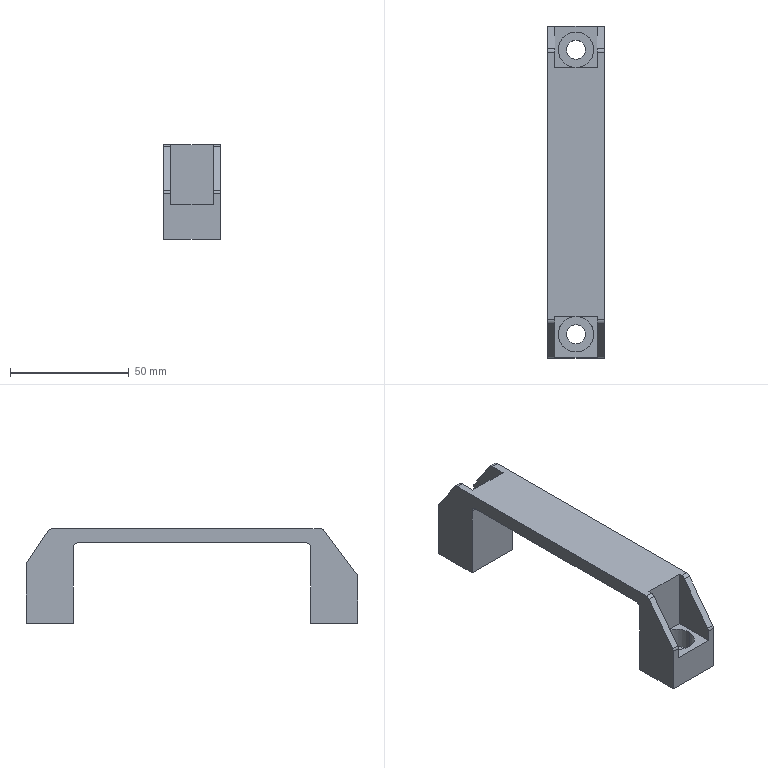Part | SolidWorks | features BaseBody 1 | 1 solid | 42 faces | box 24 x 140 x 40 mm | volume 31743 mm3 | plane 24 | cylinder 18 | commonest cylinder face diameters 4 x10 8 x4 15 x4
STEP:
#1=CARTESIAN_POINT('',(-9.,60.594,19.109));
#2=VERTEX_POINT('',#1);
#3=CARTESIAN_POINT('',(-9.,58.93,20.));
#4=VERTEX_POINT('',#3);
#5=CARTESIAN_POINT('',(-9.,58.93,18.));
#6=DIRECTION('',(1.,0.,0.));
#7=DIRECTION('',(0.,0.,1.));
#8=AXIS2_PLACEMENT_3D('',#5,#6,#7);
#9=CIRCLE('',#8,2.);
#10=EDGE_CURVE('',#2,#4,#9,.T.);
#11=ORIENTED_EDGE('',*,*,#10,.F.);
#12=CARTESIAN_POINT('',(-12.,60.594,19.109));
#13=VERTEX_POINT('',#12);
#14=CARTESIAN_POINT('',(-9.,60.594,19.109));
#15=DIRECTION('',(1.,0.,0.));
#16=VECTOR('',#15,1000.);
#17=LINE('',#14,#16);
#18=EDGE_CURVE('',#13,#2,#17,.T.);
#19=ORIENTED_EDGE('',*,*,#18,.F.);
#20=CARTESIAN_POINT('',(-12.,58.93,20.));
#21=VERTEX_POINT('',#20);
#22=CARTESIAN_POINT('',(-12.,58.93,18.));
#23=DIRECTION('',(-1.,0.,0.));
#24=DIRECTION('',(0.,0.,-1.));
#25=AXIS2_PLACEMENT_3D('',#22,#23,#24);
#26=CIRCLE('',#25,2.);
#27=EDGE_CURVE('',#21,#13,#26,.T.);
#28=ORIENTED_EDGE('',*,*,#27,.F.);
#29=CARTESIAN_POINT('',(-12.,58.93,20.));
#30=DIRECTION('',(-1.,0.,0.));
#31=VECTOR('',#30,1000.);
#32=LINE('',#29,#31);
#33=EDGE_CURVE('',#4,#21,#32,.T.);
#34=ORIENTED_EDGE('',*,*,#33,.F.);
#35=EDGE_LOOP('',(#11,#19,#28,#34));
#36=FACE_OUTER_BOUND('',#35,.T.);
#37=CARTESIAN_POINT('',(12.,58.93,18.));
#38=DIRECTION('',(-1.,0.,0.));
#39=DIRECTION('',(0.,0.,1.));
#40=AXIS2_PLACEMENT_3D('',#37,#38,#39);
#41=CYLINDRICAL_SURFACE('',#40,2.);
#42=ADVANCED_FACE('',(#36),#41,.T.);
#43=CARTESIAN_POINT('',(-12.,69.664,5.504));
#44=VERTEX_POINT('',#43);
#45=CARTESIAN_POINT('',(-12.,70.,4.394));
#46=VERTEX_POINT('',#45);
#47=CARTESIAN_POINT('',(-12.,68.,4.394));
#48=DIRECTION('',(-1.,0.,0.));
#49=DIRECTION('',(0.,0.,-1.));
#50=AXIS2_PLACEMENT_3D('',#47,#48,#49);
#51=CIRCLE('',#50,2.);
#52=EDGE_CURVE('',#44,#46,#51,.T.);
#53=ORIENTED_EDGE('',*,*,#52,.F.);
#54=CARTESIAN_POINT('',(-9.,69.664,5.504));
#55=VERTEX_POINT('',#54);
#56=CARTESIAN_POINT('',(-12.,69.664,5.504));
#57=DIRECTION('',(-1.,0.,0.));
#58=VECTOR('',#57,1000.);
#59=LINE('',#56,#58);
#60=EDGE_CURVE('',#55,#44,#59,.T.);
#61=ORIENTED_EDGE('',*,*,#60,.F.);
#62=CARTESIAN_POINT('',(-9.,70.,4.394));
#63=VERTEX_POINT('',#62);
#64=CARTESIAN_POINT('',(-9.,68.,4.394));
#65=DIRECTION('',(1.,0.,0.));
#66=DIRECTION('',(0.,0.,1.));
#67=AXIS2_PLACEMENT_3D('',#64,#65,#66);
#68=CIRCLE('',#67,2.);
#69=EDGE_CURVE('',#63,#55,#68,.T.);
#70=ORIENTED_EDGE('',*,*,#69,.F.);
#71=CARTESIAN_POINT('',(-9.,70.,4.394));
#72=DIRECTION('',(1.,0.,0.));
#73=VECTOR('',#72,1000.);
#74=LINE('',#71,#73);
#75=EDGE_CURVE('',#46,#63,#74,.T.);
#76=ORIENTED_EDGE('',*,*,#75,.F.);
#77=EDGE_LOOP('',(#53,#61,#70,#76));
#78=FACE_OUTER_BOUND('',#77,.T.);
#79=CARTESIAN_POINT('',(12.,68.,4.394));
#80=DIRECTION('',(1.,0.,0.));
#81=DIRECTION('',(0.,0.,-1.));
#82=AXIS2_PLACEMENT_3D('',#79,#80,#81);
#83=CYLINDRICAL_SURFACE('',#82,2.);
#84=ADVANCED_FACE('',(#78),#83,.T.);
#85=CARTESIAN_POINT('',(9.,69.664,5.504));
#86=VERTEX_POINT('',#85);
#87=CARTESIAN_POINT('',(9.,70.,4.394));
#88=VERTEX_POINT('',#87);
#89=CARTESIAN_POINT('',(9.,68.,4.394));
#90=DIRECTION('',(-1.,0.,0.));
#91=DIRECTION('',(0.,0.,-1.));
#92=AXIS2_PLACEMENT_3D('',#89,#90,#91);
#93=CIRCLE('',#92,2.);
#94=EDGE_CURVE('',#86,#88,#93,.T.);
#95=ORIENTED_EDGE('',*,*,#94,.F.);
#96=CARTESIAN_POINT('',(12.,69.664,5.504));
#97=VERTEX_POINT('',#96);
#98=CARTESIAN_POINT('',(9.,69.664,5.504));
#99=DIRECTION('',(-1.,0.,0.));
#100=VECTOR('',#99,1000.);
#101=LINE('',#98,#100);
#102=EDGE_CURVE('',#97,#86,#101,.T.);
#103=ORIENTED_EDGE('',*,*,#102,.F.);
#104=CARTESIAN_POINT('',(12.,70.,4.394));
#105=VERTEX_POINT('',#104);
#106=CARTESIAN_POINT('',(12.,68.,4.394));
#107=DIRECTION('',(1.,0.,0.));
#108=DIRECTION('',(0.,0.,-1.));
#109=AXIS2_PLACEMENT_3D('',#106,#107,#108);
#110=CIRCLE('',#109,2.);
#111=EDGE_CURVE('',#105,#97,#110,.T.);
#112=ORIENTED_EDGE('',*,*,#111,.F.);
#113=CARTESIAN_POINT('',(12.,70.,4.394));
#114=DIRECTION('',(1.,0.,0.));
#115=VECTOR('',#114,1000.);
#116=LINE('',#113,#115);
#117=EDGE_CURVE('',#88,#105,#116,.T.);
#118=ORIENTED_EDGE('',*,*,#117,.F.);
#119=EDGE_LOOP('',(#95,#103,#112,#118));
#120=FACE_OUTER_BOUND('',#119,.T.);
#121=CARTESIAN_POINT('',(12.,68.,4.394));
#122=DIRECTION('',(1.,0.,0.));
#123=DIRECTION('',(0.,0.,-1.));
#124=AXIS2_PLACEMENT_3D('',#121,#122,#123);
#125=CYLINDRICAL_SURFACE('',#124,2.);
#126=ADVANCED_FACE('',(#120),#125,.T.);
#127=CARTESIAN_POINT('',(9.,-55.6,19.2));
#128=VERTEX_POINT('',#127);
#129=CARTESIAN_POINT('',(9.,-54.,20.));
#130=VERTEX_POINT('',#129);
#131=CARTESIAN_POINT('',(9.,-54.,18.));
#132=DIRECTION('',(-1.,0.,0.));
#133=DIRECTION('',(0.,0.,1.));
#134=AXIS2_PLACEMENT_3D('',#131,#132,#133);
#135=CIRCLE('',#134,2.);
#136=EDGE_CURVE('',#128,#130,#135,.T.);
#137=ORIENTED_EDGE('',*,*,#136,.F.);
#138=CARTESIAN_POINT('',(12.,-55.6,19.2));
#139=VERTEX_POINT('',#138);
#140=CARTESIAN_POINT('',(9.,-55.6,19.2));
#141=DIRECTION('',(-1.,0.,0.));
#142=VECTOR('',#141,1000.);
#143=LINE('',#140,#142);
#144=EDGE_CURVE('',#139,#128,#143,.T.);
#145=ORIENTED_EDGE('',*,*,#144,.F.);
#146=CARTESIAN_POINT('',(12.,-54.,20.));
#147=VERTEX_POINT('',#146);
#148=CARTESIAN_POINT('',(12.,-54.,18.));
#149=DIRECTION('',(1.,0.,0.));
#150=DIRECTION('',(0.,0.,-1.));
#151=AXIS2_PLACEMENT_3D('',#148,#149,#150);
#152=CIRCLE('',#151,2.);
#153=EDGE_CURVE('',#147,#139,#152,.T.);
#154=ORIENTED_EDGE('',*,*,#153,.F.);
#155=CARTESIAN_POINT('',(12.,-54.,20.));
#156=DIRECTION('',(1.,0.,0.));
#157=VECTOR('',#156,1000.);
#158=LINE('',#155,#157);
#159=EDGE_CURVE('',#130,#147,#158,.T.);
#160=ORIENTED_EDGE('',*,*,#159,.F.);
#161=EDGE_LOOP('',(#137,#145,#154,#160));
#162=FACE_OUTER_BOUND('',#161,.T.);
#163=CARTESIAN_POINT('',(12.,-54.,18.));
#164=DIRECTION('',(1.,0.,0.));
#165=DIRECTION('',(0.,0.,-1.));
#166=AXIS2_PLACEMENT_3D('',#163,#164,#165);
#167=CYLINDRICAL_SURFACE('',#166,2.);
#168=ADVANCED_FACE('',(#162),#167,.T.);
#169=CARTESIAN_POINT('',(-12.,-55.6,19.2));
#170=VERTEX_POINT('',#169);
#171=CARTESIAN_POINT('',(-12.,-54.,20.));
#172=VERTEX_POINT('',#171);
#173=CARTESIAN_POINT('',(-12.,-54.,18.));
#174=DIRECTION('',(-1.,0.,0.));
#175=DIRECTION('',(0.,0.,-1.));
#176=AXIS2_PLACEMENT_3D('',#173,#174,#175);
#177=CIRCLE('',#176,2.);
#178=EDGE_CURVE('',#170,#172,#177,.T.);
#179=ORIENTED_EDGE('',*,*,#178,.F.);
#180=CARTESIAN_POINT('',(-9.,-55.6,19.2));
#181=VERTEX_POINT('',#180);
#182=CARTESIAN_POINT('',(-12.,-55.6,19.2));
#183=DIRECTION('',(-1.,0.,0.));
#184=VECTOR('',#183,1000.);
#185=LINE('',#182,#184);
#186=EDGE_CURVE('',#181,#170,#185,.T.);
#187=ORIENTED_EDGE('',*,*,#186,.F.);
#188=CARTESIAN_POINT('',(-9.,-54.,20.));
#189=VERTEX_POINT('',#188);
#190=CARTESIAN_POINT('',(-9.,-54.,18.));
#191=DIRECTION('',(1.,0.,0.));
#192=DIRECTION('',(0.,0.,-1.));
#193=AXIS2_PLACEMENT_3D('',#190,#191,#192);
#194=CIRCLE('',#193,2.);
#195=EDGE_CURVE('',#189,#181,#194,.T.);
#196=ORIENTED_EDGE('',*,*,#195,.F.);
#197=CARTESIAN_POINT('',(-9.,-54.,20.));
#198=DIRECTION('',(1.,0.,0.));
#199=VECTOR('',#198,1000.);
#200=LINE('',#197,#199);
#201=EDGE_CURVE('',#172,#189,#200,.T.);
#202=ORIENTED_EDGE('',*,*,#201,.F.);
#203=EDGE_LOOP('',(#179,#187,#196,#202));
#204=FACE_OUTER_BOUND('',#203,.T.);
#205=CARTESIAN_POINT('',(12.,-54.,18.));
#206=DIRECTION('',(1.,0.,0.));
#207=DIRECTION('',(0.,0.,-1.));
#208=AXIS2_PLACEMENT_3D('',#205,#206,#207);
#209=CYLINDRICAL_SURFACE('',#208,2.);
#210=ADVANCED_FACE('',(#204),#209,.T.);
#211=CARTESIAN_POINT('',(-9.,-69.6,0.5333));
#212=VERTEX_POINT('',#211);
#213=CARTESIAN_POINT('',(-9.,-70.,-0.6667));
#214=VERTEX_POINT('',#213);
#215=CARTESIAN_POINT('',(-9.,-68.,-0.6667));
#216=DIRECTION('',(1.,0.,0.));
#217=DIRECTION('',(0.,0.,-1.));
#218=AXIS2_PLACEMENT_3D('',#215,#216,#217);
#219=CIRCLE('',#218,2.);
#220=EDGE_CURVE('',#212,#214,#219,.T.);
#221=ORIENTED_EDGE('',*,*,#220,.F.);
#222=CARTESIAN_POINT('',(-12.,-69.6,0.5333));
#223=VERTEX_POINT('',#222);
#224=CARTESIAN_POINT('',(-9.,-69.6,0.5333));
#225=DIRECTION('',(1.,0.,0.));
#226=VECTOR('',#225,1000.);
#227=LINE('',#224,#226);
#228=EDGE_CURVE('',#223,#212,#227,.T.);
#229=ORIENTED_EDGE('',*,*,#228,.F.);
#230=CARTESIAN_POINT('',(-12.,-70.,-0.6667));
#231=VERTEX_POINT('',#230);
#232=CARTESIAN_POINT('',(-12.,-68.,-0.6667));
#233=DIRECTION('',(-1.,0.,0.));
#234=DIRECTION('',(0.,0.,-1.));
#235=AXIS2_PLACEMENT_3D('',#232,#233,#234);
#236=CIRCLE('',#235,2.);
#237=EDGE_CURVE('',#231,#223,#236,.T.);
#238=ORIENTED_EDGE('',*,*,#237,.F.);
#239=CARTESIAN_POINT('',(-12.,-70.,-0.6667));
#240=DIRECTION('',(-1.,0.,0.));
#241=VECTOR('',#240,1000.);
#242=LINE('',#239,#241);
#243=EDGE_CURVE('',#214,#231,#242,.T.);
#244=ORIENTED_EDGE('',*,*,#243,.F.);
#245=EDGE_LOOP('',(#221,#229,#238,#244));
#246=FACE_OUTER_BOUND('',#245,.T.);
#247=CARTESIAN_POINT('',(12.,-68.,-0.6667));
#248=DIRECTION('',(-1.,0.,0.));
#249=DIRECTION('',(0.,0.,1.));
#250=AXIS2_PLACEMENT_3D('',#247,#248,#249);
#251=CYLINDRICAL_SURFACE('',#250,2.);
#252=ADVANCED_FACE('',(#246),#251,.T.);
#253=CARTESIAN_POINT('',(12.,-69.6,0.5333));
#254=VERTEX_POINT('',#253);
#255=CARTESIAN_POINT('',(12.,-70.,-0.6667));
#256=VERTEX_POINT('',#255);
#257=CARTESIAN_POINT('',(12.,-68.,-0.6667));
#258=DIRECTION('',(1.,0.,0.));
#259=DIRECTION('',(0.,0.,-1.));
#260=AXIS2_PLACEMENT_3D('',#257,#258,#259);
#261=CIRCLE('',#260,2.);
#262=EDGE_CURVE('',#254,#256,#261,.T.);
#263=ORIENTED_EDGE('',*,*,#262,.F.);
#264=CARTESIAN_POINT('',(9.,-69.6,0.5333));
#265=VERTEX_POINT('',#264);
#266=CARTESIAN_POINT('',(12.,-69.6,0.5333));
#267=DIRECTION('',(1.,0.,0.));
#268=VECTOR('',#267,1000.);
#269=LINE('',#266,#268);
#270=EDGE_CURVE('',#265,#254,#269,.T.);
#271=ORIENTED_EDGE('',*,*,#270,.F.);
#272=CARTESIAN_POINT('',(9.,-70.,-0.6667));
#273=VERTEX_POINT('',#272);
#274=CARTESIAN_POINT('',(9.,-68.,-0.6667));
#275=DIRECTION('',(-1.,0.,0.));
#276=DIRECTION('',(0.,0.,1.));
#277=AXIS2_PLACEMENT_3D('',#274,#275,#276);
#278=CIRCLE('',#277,2.);
#279=EDGE_CURVE('',#273,#265,#278,.T.);
#280=ORIENTED_EDGE('',*,*,#279,.F.);
#281=CARTESIAN_POINT('',(9.,-70.,-0.6667));
#282=DIRECTION('',(-1.,0.,0.));
#283=VECTOR('',#282,1000.);
#284=LINE('',#281,#283);
#285=EDGE_CURVE('',#256,#273,#284,.T.);
#286=ORIENTED_EDGE('',*,*,#285,.F.);
#287=EDGE_LOOP('',(#263,#271,#280,#286));
#288=FACE_OUTER_BOUND('',#287,.T.);
#289=CARTESIAN_POINT('',(12.,-68.,-0.6667));
#290=DIRECTION('',(-1.,0.,0.));
#291=DIRECTION('',(0.,0.,1.));
#292=AXIS2_PLACEMENT_3D('',#289,#290,#291);
#293=CYLINDRICAL_SURFACE('',#292,2.);
#294=ADVANCED_FACE('',(#288),#293,.T.);
#295=CARTESIAN_POINT('',(-12.,50.,12.));
#296=VERTEX_POINT('',#295);
#297=CARTESIAN_POINT('',(-12.,48.,14.));
#298=VERTEX_POINT('',#297);
#299=CARTESIAN_POINT('',(-12.,48.,12.));
#300=DIRECTION('',(1.,0.,0.));
#301=DIRECTION('',(0.,0.,-1.));
#302=AXIS2_PLACEMENT_3D('',#299,#300,#301);
#303=CIRCLE('',#302,2.);
#304=EDGE_CURVE('',#296,#298,#303,.T.);
#305=ORIENTED_EDGE('',*,*,#304,.F.);
#306=CARTESIAN_POINT('',(12.,50.,12.));
#307=VERTEX_POINT('',#306);
#308=CARTESIAN_POINT('',(-12.,50.,12.));
#309=DIRECTION('',(-1.,0.,0.));
#310=VECTOR('',#309,1000.);
#311=LINE('',#308,#310);
#312=EDGE_CURVE('',#307,#296,#311,.T.);
#313=ORIENTED_EDGE('',*,*,#312,.F.);
#314=CARTESIAN_POINT('',(12.,48.,14.));
#315=VERTEX_POINT('',#314);
#316=CARTESIAN_POINT('',(12.,48.,12.));
#317=DIRECTION('',(-1.,0.,0.));
#318=DIRECTION('',(0.,0.,-1.));
#319=AXIS2_PLACEMENT_3D('',#316,#317,#318);
#320=CIRCLE('',#319,2.);
#321=EDGE_CURVE('',#315,#307,#320,.T.);
#322=ORIENTED_EDGE('',*,*,#321,.F.);
#323=CARTESIAN_POINT('',(12.,48.,14.));
#324=DIRECTION('',(1.,0.,0.));
#325=VECTOR('',#324,1000.);
#326=LINE('',#323,#325);
#327=EDGE_CURVE('',#298,#315,#326,.T.);
#328=ORIENTED_EDGE('',*,*,#327,.F.);
#329=EDGE_LOOP('',(#305,#313,#322,#328));
#330=FACE_OUTER_BOUND('',#329,.T.);
#331=CARTESIAN_POINT('',(-12.,48.,12.));
#332=DIRECTION('',(-1.,0.,0.));
#333=DIRECTION('',(0.,0.,1.));
#334=AXIS2_PLACEMENT_3D('',#331,#332,#333);
#335=CYLINDRICAL_SURFACE('',#334,2.);
#336=ADVANCED_FACE('',(#330),#335,.F.);
#337=CARTESIAN_POINT('',(-12.,-48.,14.));
#338=VERTEX_POINT('',#337);
#339=CARTESIAN_POINT('',(-12.,-50.,12.));
#340=VERTEX_POINT('',#339);
#341=CARTESIAN_POINT('',(-12.,-48.,12.));
#342=DIRECTION('',(1.,0.,0.));
#343=DIRECTION('',(0.,0.,-1.));
#344=AXIS2_PLACEMENT_3D('',#341,#342,#343);
#345=CIRCLE('',#344,2.);
#346=EDGE_CURVE('',#338,#340,#345,.T.);
#347=ORIENTED_EDGE('',*,*,#346,.F.);
#348=CARTESIAN_POINT('',(12.,-48.,14.));
#349=VERTEX_POINT('',#348);
#350=CARTESIAN_POINT('',(-12.,-48.,14.));
#351=DIRECTION('',(-1.,0.,0.));
#352=VECTOR('',#351,1000.);
#353=LINE('',#350,#352);
#354=EDGE_CURVE('',#349,#338,#353,.T.);
#355=ORIENTED_EDGE('',*,*,#354,.F.);
#356=CARTESIAN_POINT('',(12.,-50.,12.));
#357=VERTEX_POINT('',#356);
#358=CARTESIAN_POINT('',(12.,-48.,12.));
#359=DIRECTION('',(-1.,0.,0.));
#360=DIRECTION('',(0.,0.,-1.));
#361=AXIS2_PLACEMENT_3D('',#358,#359,#360);
#362=CIRCLE('',#361,2.);
#363=EDGE_CURVE('',#357,#349,#362,.T.);
#364=ORIENTED_EDGE('',*,*,#363,.F.);
#365=CARTESIAN_POINT('',(12.,-50.,12.));
#366=DIRECTION('',(1.,0.,0.));
#367=VECTOR('',#366,1000.);
#368=LINE('',#365,#367);
#369=EDGE_CURVE('',#340,#357,#368,.T.);
#370=ORIENTED_EDGE('',*,*,#369,.F.);
#371=EDGE_LOOP('',(#347,#355,#364,#370));
#372=FACE_OUTER_BOUND('',#371,.T.);
#373=CARTESIAN_POINT('',(-12.,-48.,12.));
#374=DIRECTION('',(-1.,0.,0.));
#375=DIRECTION('',(0.,0.,1.));
#376=AXIS2_PLACEMENT_3D('',#373,#374,#375);
#377=CYLINDRICAL_SURFACE('',#376,2.);
#378=ADVANCED_FACE('',(#372),#377,.F.);
#379=CARTESIAN_POINT('',(12.,60.594,19.109));
#380=VERTEX_POINT('',#379);
#381=CARTESIAN_POINT('',(12.,58.93,20.));
#382=VERTEX_POINT('',#381);
#383=CARTESIAN_POINT('',(12.,58.93,18.));
#384=DIRECTION('',(1.,0.,0.));
#385=DIRECTION('',(0.,0.,-1.));
#386=AXIS2_PLACEMENT_3D('',#383,#384,#385);
#387=CIRCLE('',#386,2.);
#388=EDGE_CURVE('',#380,#382,#387,.T.);
#389=ORIENTED_EDGE('',*,*,#388,.F.);
#390=CARTESIAN_POINT('',(9.,60.594,19.109));
#391=VERTEX_POINT('',#390);
#392=CARTESIAN_POINT('',(12.,60.594,19.109));
#393=DIRECTION('',(1.,0.,0.));
#394=VECTOR('',#393,1000.);
#395=LINE('',#392,#394);
#396=EDGE_CURVE('',#391,#380,#395,.T.);
#397=ORIENTED_EDGE('',*,*,#396,.F.);
#398=CARTESIAN_POINT('',(9.,58.93,20.));
#399=VERTEX_POINT('',#398);
#400=CARTESIAN_POINT('',(9.,58.93,18.));
#401=DIRECTION('',(-1.,0.,0.));
#402=DIRECTION('',(0.,0.,-1.));
#403=AXIS2_PLACEMENT_3D('',#400,#401,#402);
#404=CIRCLE('',#403,2.);
#405=EDGE_CURVE('',#399,#391,#404,.T.);
#406=ORIENTED_EDGE('',*,*,#405,.F.);
#407=CARTESIAN_POINT('',(9.,58.93,20.));
#408=DIRECTION('',(-1.,0.,0.));
#409=VECTOR('',#408,1000.);
#410=LINE('',#407,#409);
#411=EDGE_CURVE('',#382,#399,#410,.T.);
#412=ORIENTED_EDGE('',*,*,#411,.F.);
#413=EDGE_LOOP('',(#389,#397,#406,#412));
#414=FACE_OUTER_BOUND('',#413,.T.);
#415=CARTESIAN_POINT('',(12.,58.93,18.));
#416=DIRECTION('',(-1.,0.,0.));
#417=DIRECTION('',(0.,0.,1.));
#418=AXIS2_PLACEMENT_3D('',#415,#416,#417);
#419=CYLINDRICAL_SURFACE('',#418,2.);
#420=ADVANCED_FACE('',(#414),#419,.T.);
#421=CARTESIAN_POINT('',(-7.5,-60.,-14.4));
#422=VERTEX_POINT('',#421);
#423=CARTESIAN_POINT('',(-7.5,-60.,-5.4));
#424=VERTEX_POINT('',#423);
#425=CARTESIAN_POINT('',(-7.5,-60.,-14.4));
#426=DIRECTION('',(0.,0.,1.));
#427=VECTOR('',#426,1000.);
#428=LINE('',#425,#427);
#429=EDGE_CURVE('',#422,#424,#428,.T.);
#430=ORIENTED_EDGE('',*,*,#429,.F.);
#431=CARTESIAN_POINT('',(7.5,-60.,-14.4));
#432=VERTEX_POINT('',#431);
#433=CARTESIAN_POINT('',(0.,-60.,-14.4));
#434=DIRECTION('',(0.,0.,1.));
#435=DIRECTION('',(1.,0.,0.));
#436=AXIS2_PLACEMENT_3D('',#433,#434,#435);
#437=CIRCLE('',#436,7.5);
#438=EDGE_CURVE('',#432,#422,#437,.T.);
#439=ORIENTED_EDGE('',*,*,#438,.F.);
#440=CARTESIAN_POINT('',(7.5,-60.,-5.4));
#441=VERTEX_POINT('',#440);
#442=CARTESIAN_POINT('',(7.5,-60.,-14.4));
#443=DIRECTION('',(0.,0.,1.));
#444=VECTOR('',#443,1000.);
#445=LINE('',#442,#444);
#446=EDGE_CURVE('',#432,#441,#445,.T.);
#447=ORIENTED_EDGE('',*,*,#446,.T.);
#448=CARTESIAN_POINT('',(0.,-52.5,-5.4));
#449=VERTEX_POINT('',#448);
#450=CARTESIAN_POINT('',(0.,-60.,-5.4));
#451=DIRECTION('',(0.,0.,1.));
#452=DIRECTION('',(1.,0.,0.));
#453=AXIS2_PLACEMENT_3D('',#450,#451,#452);
#454=CIRCLE('',#453,7.5);
#455=EDGE_CURVE('',#441,#449,#454,.T.);
#456=ORIENTED_EDGE('',*,*,#455,.T.);
#457=CARTESIAN_POINT('',(0.,-60.,-5.4));
#458=DIRECTION('',(0.,0.,1.));
#459=DIRECTION('',(1.,0.,0.));
#460=AXIS2_PLACEMENT_3D('',#457,#458,#459);
#461=CIRCLE('',#460,7.5);
#462=EDGE_CURVE('',#449,#424,#461,.T.);
#463=ORIENTED_EDGE('',*,*,#462,.T.);
#464=EDGE_LOOP('',(#430,#439,#447,#456,#463));
#465=FACE_OUTER_BOUND('',#464,.T.);
#466=CARTESIAN_POINT('',(0.,-60.,-14.4));
#467=DIRECTION('',(0.,0.,1.));
#468=DIRECTION('',(1.,0.,0.));
#469=AXIS2_PLACEMENT_3D('',#466,#467,#468);
#470=CYLINDRICAL_SURFACE('',#469,7.5);
#471=ADVANCED_FACE('',(#465),#470,.F.);
#472=CARTESIAN_POINT('',(0.,-56.,-14.4));
#473=VERTEX_POINT('',#472);
#474=CARTESIAN_POINT('',(0.,-64.,-14.4));
#475=VERTEX_POINT('',#474);
#476=CARTESIAN_POINT('',(0.,-60.,-14.4));
#477=DIRECTION('',(0.,0.,-1.));
#478=DIRECTION('',(1.,0.,0.));
#479=AXIS2_PLACEMENT_3D('',#476,#477,#478);
#480=CIRCLE('',#479,4.);
#481=EDGE_CURVE('',#473,#475,#480,.T.);
#482=ORIENTED_EDGE('',*,*,#481,.T.);
#483=CARTESIAN_POINT('',(0.,-60.,-14.4));
#484=DIRECTION('',(0.,0.,-1.));
#485=DIRECTION('',(1.,0.,0.));
#486=AXIS2_PLACEMENT_3D('',#483,#484,#485);
#487=CIRCLE('',#486,4.);
#488=EDGE_CURVE('',#475,#473,#487,.T.);
#489=ORIENTED_EDGE('',*,*,#488,.T.);
#490=EDGE_LOOP('',(#482,#489));
#491=FACE_BOUND('',#490,.T.);
#492=ORIENTED_EDGE('',*,*,#438,.T.);
#493=CARTESIAN_POINT('',(0.,-60.,-14.4));
#494=DIRECTION('',(0.,0.,1.));
#495=DIRECTION('',(1.,0.,0.));
#496=AXIS2_PLACEMENT_3D('',#493,#494,#495);
#497=CIRCLE('',#496,7.5);
#498=EDGE_CURVE('',#422,#432,#497,.T.);
#499=ORIENTED_EDGE('',*,*,#498,.T.);
#500=EDGE_LOOP('',(#492,#499));
#501=FACE_OUTER_BOUND('',#500,.T.);
#502=CARTESIAN_POINT('',(0.,-60.,-14.4));
#503=DIRECTION('',(0.,0.,1.));
#504=DIRECTION('',(1.,0.,0.));
#505=AXIS2_PLACEMENT_3D('',#502,#503,#504);
#506=PLANE('',#505);
#507=ADVANCED_FACE('',(#491,#501),#506,.T.);
#508=CARTESIAN_POINT('',(-7.5,60.,-14.4));
#509=VERTEX_POINT('',#508);
#510=CARTESIAN_POINT('',(-7.5,60.,-5.4));
#511=VERTEX_POINT('',#510);
#512=CARTESIAN_POINT('',(-7.5,60.,-14.4));
#513=DIRECTION('',(0.,0.,1.));
#514=VECTOR('',#513,1000.);
#515=LINE('',#512,#514);
#516=EDGE_CURVE('',#509,#511,#515,.T.);
#517=ORIENTED_EDGE('',*,*,#516,.F.);
#518=CARTESIAN_POINT('',(7.5,60.,-14.4));
#519=VERTEX_POINT('',#518);
#520=CARTESIAN_POINT('',(0.,60.,-14.4));
#521=DIRECTION('',(0.,0.,1.));
#522=DIRECTION('',(1.,0.,0.));
#523=AXIS2_PLACEMENT_3D('',#520,#521,#522);
#524=CIRCLE('',#523,7.5);
#525=EDGE_CURVE('',#519,#509,#524,.T.);
#526=ORIENTED_EDGE('',*,*,#525,.F.);
#527=CARTESIAN_POINT('',(7.5,60.,-5.4));
#528=VERTEX_POINT('',#527);
#529=CARTESIAN_POINT('',(7.5,60.,-14.4));
#530=DIRECTION('',(0.,0.,1.));
#531=VECTOR('',#530,1000.);
#532=LINE('',#529,#531);
#533=EDGE_CURVE('',#519,#528,#532,.T.);
#534=ORIENTED_EDGE('',*,*,#533,.T.);
#535=CARTESIAN_POINT('',(0.,60.,-5.4));
#536=DIRECTION('',(0.,0.,1.));
#537=DIRECTION('',(1.,0.,0.));
#538=AXIS2_PLACEMENT_3D('',#535,#536,#537);
#539=CIRCLE('',#538,7.5);
#540=EDGE_CURVE('',#528,#511,#539,.T.);
#541=ORIENTED_EDGE('',*,*,#540,.T.);
#542=EDGE_LOOP('',(#517,#526,#534,#541));
#543=FACE_OUTER_BOUND('',#542,.T.);
#544=CARTESIAN_POINT('',(0.,60.,-14.4));
#545=DIRECTION('',(0.,0.,1.));
#546=DIRECTION('',(1.,0.,0.));
#547=AXIS2_PLACEMENT_3D('',#544,#545,#546);
#548=CYLINDRICAL_SURFACE('',#547,7.5);
#549=ADVANCED_FACE('',(#543),#548,.F.);
#550=CARTESIAN_POINT('',(0.,64.,-14.4));
#551=VERTEX_POINT('',#550);
#552=CARTESIAN_POINT('',(0.,56.,-14.4));
#553=VERTEX_POINT('',#552);
#554=CARTESIAN_POINT('',(0.,60.,-14.4));
#555=DIRECTION('',(0.,0.,-1.));
#556=DIRECTION('',(1.,0.,0.));
#557=AXIS2_PLACEMENT_3D('',#554,#555,#556);
#558=CIRCLE('',#557,4.);
#559=EDGE_CURVE('',#551,#553,#558,.T.);
#560=ORIENTED_EDGE('',*,*,#559,.T.);
#561=CARTESIAN_POINT('',(0.,60.,-14.4));
#562=DIRECTION('',(0.,0.,-1.));
#563=DIRECTION('',(1.,0.,0.));
#564=AXIS2_PLACEMENT_3D('',#561,#562,#563);
#565=CIRCLE('',#564,4.);
#566=EDGE_CURVE('',#553,#551,#565,.T.);
#567=ORIENTED_EDGE('',*,*,#566,.T.);
#568=EDGE_LOOP('',(#560,#567));
#569=FACE_BOUND('',#568,.T.);
#570=ORIENTED_EDGE('',*,*,#525,.T.);
#571=CARTESIAN_POINT('',(0.,60.,-14.4));
#572=DIRECTION('',(0.,0.,1.));
#573=DIRECTION('',(1.,0.,0.));
#574=AXIS2_PLACEMENT_3D('',#571,#572,#573);
#575=CIRCLE('',#574,7.5);
#576=EDGE_CURVE('',#509,#519,#575,.T.);
#577=ORIENTED_EDGE('',*,*,#576,.T.);
#578=EDGE_LOOP('',(#570,#577));
#579=FACE_OUTER_BOUND('',#578,.T.);
#580=CARTESIAN_POINT('',(0.,60.,-14.4));
#581=DIRECTION('',(0.,0.,1.));
#582=DIRECTION('',(1.,0.,0.));
#583=AXIS2_PLACEMENT_3D('',#580,#581,#582);
#584=PLANE('',#583);
#585=ADVANCED_FACE('',(#569,#579),#584,.T.);
#586=CARTESIAN_POINT('',(9.,-52.5,-5.4));
#587=VERTEX_POINT('',#586);
#588=CARTESIAN_POINT('',(9.,-52.5,-5.4));
#589=DIRECTION('',(-1.,0.,0.));
#590=VECTOR('',#589,1000.);
#591=LINE('',#588,#590);
#592=EDGE_CURVE('',#587,#449,#591,.T.);
#593=ORIENTED_EDGE('',*,*,#592,.T.);
#594=ORIENTED_EDGE('',*,*,#455,.F.);
#595=CARTESIAN_POINT('',(0.,-60.,-5.4));
#596=DIRECTION('',(0.,0.,1.));
#597=DIRECTION('',(1.,0.,0.));
#598=AXIS2_PLACEMENT_3D('',#595,#596,#597);
#599=CIRCLE('',#598,7.5);
#600=EDGE_CURVE('',#424,#441,#599,.T.);
#601=ORIENTED_EDGE('',*,*,#600,.F.);
#602=ORIENTED_EDGE('',*,*,#462,.F.);
#603=CARTESIAN_POINT('',(-9.,-52.5,-5.4));
#604=VERTEX_POINT('',#603);
#605=CARTESIAN_POINT('',(9.,-52.5,-5.4));
#606=DIRECTION('',(-1.,0.,0.));
#607=VECTOR('',#606,1000.);
#608=LINE('',#605,#607);
#609=EDGE_CURVE('',#449,#604,#608,.T.);
#610=ORIENTED_EDGE('',*,*,#609,.T.);
#611=CARTESIAN_POINT('',(-9.,-70.,-5.4));
#612=VERTEX_POINT('',#611);
#613=CARTESIAN_POINT('',(-9.,-52.5,-5.4));
#614=DIRECTION('',(0.,-1.,0.));
#615=VECTOR('',#614,1000.);
#616=LINE('',#613,#615);
#617=EDGE_CURVE('',#604,#612,#616,.T.);
#618=ORIENTED_EDGE('',*,*,#617,.T.);
#619=CARTESIAN_POINT('',(9.,-70.,-5.4));
#620=VERTEX_POINT('',#619);
#621=CARTESIAN_POINT('',(9.,-70.,-5.4));
#622=DIRECTION('',(1.,0.,0.));
#623=VECTOR('',#622,1000.);
#624=LINE('',#621,#623);
#625=EDGE_CURVE('',#612,#620,#624,.T.);
#626=ORIENTED_EDGE('',*,*,#625,.T.);
#627=CARTESIAN_POINT('',(9.,-52.5,-5.4));
#628=DIRECTION('',(0.,1.,0.));
#629=VECTOR('',#628,1000.);
#630=LINE('',#627,#629);
#631=EDGE_CURVE('',#620,#587,#630,.T.);
#632=ORIENTED_EDGE('',*,*,#631,.T.);
#633=EDGE_LOOP('',(#593,#594,#601,#602,#610,#618,#626,#632));
#634=FACE_OUTER_BOUND('',#633,.T.);
#635=CARTESIAN_POINT('',(12.,70.,-5.4));
#636=DIRECTION('',(0.,0.,1.));
#637=DIRECTION('',(0.,-1.,0.));
#638=AXIS2_PLACEMENT_3D('',#635,#636,#637);
#639=PLANE('',#638);
#640=ADVANCED_FACE('',(#634),#639,.T.);
#641=CARTESIAN_POINT('',(-9.,-70.,0.));
#642=DIRECTION('',(0.,0.6,0.8));
#643=VECTOR('',#642,1000.);
#644=LINE('',#641,#643);
#645=EDGE_CURVE('',#212,#181,#644,.T.);
#646=ORIENTED_EDGE('',*,*,#645,.F.);
#647=ORIENTED_EDGE('',*,*,#220,.T.);
#648=CARTESIAN_POINT('',(-9.,-70.,-45.105));
#649=DIRECTION('',(0.,0.,1.));
#650=VECTOR('',#649,1000.);
#651=LINE('',#648,#650);
#652=EDGE_CURVE('',#612,#214,#651,.T.);
#653=ORIENTED_EDGE('',*,*,#652,.F.);
#654=ORIENTED_EDGE('',*,*,#617,.F.);
#655=CARTESIAN_POINT('',(-9.,-52.5,20.));
#656=VERTEX_POINT('',#655);
#657=CARTESIAN_POINT('',(-9.,-52.5,-45.105));
#658=DIRECTION('',(0.,0.,1.));
#659=VECTOR('',#658,1000.);
#660=LINE('',#657,#659);
#661=EDGE_CURVE('',#604,#656,#660,.T.);
#662=ORIENTED_EDGE('',*,*,#661,.T.);
#663=CARTESIAN_POINT('',(-9.,-52.5,20.));
#664=DIRECTION('',(0.,1.,0.));
#665=VECTOR('',#664,1000.);
#666=LINE('',#663,#665);
#667=EDGE_CURVE('',#189,#656,#666,.T.);
#668=ORIENTED_EDGE('',*,*,#667,.F.);
#669=ORIENTED_EDGE('',*,*,#195,.T.);
#670=EDGE_LOOP('',(#646,#647,#653,#654,#662,#668,#669));
#671=FACE_OUTER_BOUND('',#670,.T.);
#672=CARTESIAN_POINT('',(-9.,-52.5,-45.105));
#673=DIRECTION('',(1.,0.,0.));
#674=DIRECTION('',(0.,1.,0.));
#675=AXIS2_PLACEMENT_3D('',#672,#673,#674);
#676=PLANE('',#675);
#677=ADVANCED_FACE('',(#671),#676,.T.);
#678=CARTESIAN_POINT('',(9.,-52.5,20.));
#679=VERTEX_POINT('',#678);
#680=CARTESIAN_POINT('',(9.,-52.5,-45.105));
#681=DIRECTION('',(0.,0.,1.));
#682=VECTOR('',#681,1000.);
#683=LINE('',#680,#682);
#684=EDGE_CURVE('',#587,#679,#683,.T.);
#685=ORIENTED_EDGE('',*,*,#684,.T.);
#686=CARTESIAN_POINT('',(9.,-52.5,20.));
#687=DIRECTION('',(1.,0.,0.));
#688=VECTOR('',#687,1000.);
#689=LINE('',#686,#688);
#690=EDGE_CURVE('',#656,#679,#689,.T.);
#691=ORIENTED_EDGE('',*,*,#690,.F.);
#692=ORIENTED_EDGE('',*,*,#661,.F.);
#693=ORIENTED_EDGE('',*,*,#609,.F.);
#694=ORIENTED_EDGE('',*,*,#592,.F.);
#695=EDGE_LOOP('',(#685,#691,#692,#693,#694));
#696=FACE_OUTER_BOUND('',#695,.T.);
#697=CARTESIAN_POINT('',(9.,-52.5,-45.105));
#698=DIRECTION('',(0.,-1.,0.));
#699=DIRECTION('',(0.,0.,-1.));
#700=AXIS2_PLACEMENT_3D('',#697,#698,#699);
#701=PLANE('',#700);
#702=ADVANCED_FACE('',(#696),#701,.T.);
#703=CARTESIAN_POINT('',(9.,-70.,-45.105));
#704=DIRECTION('',(0.,0.,1.));
#705=VECTOR('',#704,1000.);
#706=LINE('',#703,#705);
#707=EDGE_CURVE('',#620,#273,#706,.T.);
#708=ORIENTED_EDGE('',*,*,#707,.T.);
#709=ORIENTED_EDGE('',*,*,#279,.T.);
#710=CARTESIAN_POINT('',(9.,-70.,0.));
#711=DIRECTION('',(0.,-0.6,-0.8));
#712=VECTOR('',#711,1000.);
#713=LINE('',#710,#712);
#714=EDGE_CURVE('',#128,#265,#713,.T.);
#715=ORIENTED_EDGE('',*,*,#714,.F.);
#716=ORIENTED_EDGE('',*,*,#136,.T.);
#717=CARTESIAN_POINT('',(9.,-52.5,20.));
#718=DIRECTION('',(0.,-1.,0.));
#719=VECTOR('',#718,1000.);
#720=LINE('',#717,#719);
#721=EDGE_CURVE('',#679,#130,#720,.T.);
#722=ORIENTED_EDGE('',*,*,#721,.F.);
#723=ORIENTED_EDGE('',*,*,#684,.F.);
#724=ORIENTED_EDGE('',*,*,#631,.F.);
#725=EDGE_LOOP('',(#708,#709,#715,#716,#722,#723,#724));
#726=FACE_OUTER_BOUND('',#725,.T.);
#727=CARTESIAN_POINT('',(9.,-52.5,-45.105));
#728=DIRECTION('',(-1.,0.,0.));
#729=DIRECTION('',(0.,0.,1.));
#730=AXIS2_PLACEMENT_3D('',#727,#728,#729);
#731=PLANE('',#730);
#732=ADVANCED_FACE('',(#726),#731,.T.);
#733=CARTESIAN_POINT('',(0.,52.5,-5.4));
#734=VERTEX_POINT('',#733);
#735=CARTESIAN_POINT('',(-9.,52.5,-5.4));
#736=VERTEX_POINT('',#735);
#737=CARTESIAN_POINT('',(9.,52.5,-5.4));
#738=DIRECTION('',(-1.,0.,0.));
#739=VECTOR('',#738,1000.);
#740=LINE('',#737,#739);
#741=EDGE_CURVE('',#734,#736,#740,.T.);
#742=ORIENTED_EDGE('',*,*,#741,.F.);
#743=CARTESIAN_POINT('',(0.,60.,-5.4));
#744=DIRECTION('',(0.,0.,1.));
#745=DIRECTION('',(1.,0.,0.));
#746=AXIS2_PLACEMENT_3D('',#743,#744,#745);
#747=CIRCLE('',#746,7.5);
#748=EDGE_CURVE('',#511,#734,#747,.T.);
#749=ORIENTED_EDGE('',*,*,#748,.F.);
#750=ORIENTED_EDGE('',*,*,#540,.F.);
#751=CARTESIAN_POINT('',(0.,60.,-5.4));
#752=DIRECTION('',(0.,0.,1.));
#753=DIRECTION('',(1.,0.,0.));
#754=AXIS2_PLACEMENT_3D('',#751,#752,#753);
#755=CIRCLE('',#754,7.5);
#756=EDGE_CURVE('',#734,#528,#755,.T.);
#757=ORIENTED_EDGE('',*,*,#756,.F.);
#758=CARTESIAN_POINT('',(9.,52.5,-5.4));
#759=VERTEX_POINT('',#758);
#760=CARTESIAN_POINT('',(9.,52.5,-5.4));
#761=DIRECTION('',(-1.,0.,0.));
#762=VECTOR('',#761,1000.);
#763=LINE('',#760,#762);
#764=EDGE_CURVE('',#759,#734,#763,.T.);
#765=ORIENTED_EDGE('',*,*,#764,.F.);
#766=CARTESIAN_POINT('',(9.,70.,-5.4));
#767=VERTEX_POINT('',#766);
#768=CARTESIAN_POINT('',(9.,52.5,-5.4));
#769=DIRECTION('',(0.,-1.,0.));
#770=VECTOR('',#769,1000.);
#771=LINE('',#768,#770);
#772=EDGE_CURVE('',#767,#759,#771,.T.);
#773=ORIENTED_EDGE('',*,*,#772,.F.);
#774=CARTESIAN_POINT('',(-9.,70.,-5.4));
#775=VERTEX_POINT('',#774);
#776=CARTESIAN_POINT('',(9.,70.,-5.4));
#777=DIRECTION('',(1.,0.,0.));
#778=VECTOR('',#777,1000.);
#779=LINE('',#776,#778);
#780=EDGE_CURVE('',#775,#767,#779,.T.);
#781=ORIENTED_EDGE('',*,*,#780,.F.);
#782=CARTESIAN_POINT('',(-9.,52.5,-5.4));
#783=DIRECTION('',(0.,1.,0.));
#784=VECTOR('',#783,1000.);
#785=LINE('',#782,#784);
#786=EDGE_CURVE('',#736,#775,#785,.T.);
#787=ORIENTED_EDGE('',*,*,#786,.F.);
#788=EDGE_LOOP('',(#742,#749,#750,#757,#765,#773,#781,#787));
#789=FACE_OUTER_BOUND('',#788,.T.);
#790=CARTESIAN_POINT('',(12.,70.,-5.4));
#791=DIRECTION('',(0.,0.,1.));
#792=DIRECTION('',(0.,-1.,0.));
#793=AXIS2_PLACEMENT_3D('',#790,#791,#792);
#794=PLANE('',#793);
#795=ADVANCED_FACE('',(#789),#794,.T.);
#796=ORIENTED_EDGE('',*,*,#764,.T.);
#797=ORIENTED_EDGE('',*,*,#741,.T.);
#798=CARTESIAN_POINT('',(-9.,52.5,20.));
#799=VERTEX_POINT('',#798);
#800=CARTESIAN_POINT('',(-9.,52.5,-45.105));
#801=DIRECTION('',(0.,0.,1.));
#802=VECTOR('',#801,1000.);
#803=LINE('',#800,#802);
#804=EDGE_CURVE('',#736,#799,#803,.T.);
#805=ORIENTED_EDGE('',*,*,#804,.T.);
#806=CARTESIAN_POINT('',(9.,52.5,20.));
#807=VERTEX_POINT('',#806);
#808=CARTESIAN_POINT('',(9.,52.5,20.));
#809=DIRECTION('',(1.,0.,0.));
#810=VECTOR('',#809,1000.);
#811=LINE('',#808,#810);
#812=EDGE_CURVE('',#799,#807,#811,.T.);
#813=ORIENTED_EDGE('',*,*,#812,.T.);
#814=CARTESIAN_POINT('',(9.,52.5,-45.105));
#815=DIRECTION('',(0.,0.,1.));
#816=VECTOR('',#815,1000.);
#817=LINE('',#814,#816);
#818=EDGE_CURVE('',#759,#807,#817,.T.);
#819=ORIENTED_EDGE('',*,*,#818,.F.);
#820=EDGE_LOOP('',(#796,#797,#805,#813,#819));
#821=FACE_OUTER_BOUND('',#820,.T.);
#822=CARTESIAN_POINT('',(9.,52.5,-45.105));
#823=DIRECTION('',(0.,-1.,0.));
#824=DIRECTION('',(0.,0.,-1.));
#825=AXIS2_PLACEMENT_3D('',#822,#823,#824);
#826=PLANE('',#825);
#827=ADVANCED_FACE('',(#821),#826,.F.);
#828=CARTESIAN_POINT('',(9.,60.,20.));
#829=DIRECTION('',(0.,0.5547,-0.8321));
#830=VECTOR('',#829,1000.);
#831=LINE('',#828,#830);
#832=EDGE_CURVE('',#391,#86,#831,.T.);
#833=ORIENTED_EDGE('',*,*,#832,.T.);
#834=ORIENTED_EDGE('',*,*,#94,.T.);
#835=CARTESIAN_POINT('',(9.,70.,-45.105));
#836=DIRECTION('',(0.,0.,1.));
#837=VECTOR('',#836,1000.);
#838=LINE('',#835,#837);
#839=EDGE_CURVE('',#767,#88,#838,.T.);
#840=ORIENTED_EDGE('',*,*,#839,.F.);
#841=ORIENTED_EDGE('',*,*,#772,.T.);
#842=ORIENTED_EDGE('',*,*,#818,.T.);
#843=CARTESIAN_POINT('',(9.,52.5,20.));
#844=DIRECTION('',(0.,1.,0.));
#845=VECTOR('',#844,1000.);
#846=LINE('',#843,#845);
#847=EDGE_CURVE('',#807,#399,#846,.T.);
#848=ORIENTED_EDGE('',*,*,#847,.T.);
#849=ORIENTED_EDGE('',*,*,#405,.T.);
#850=EDGE_LOOP('',(#833,#834,#840,#841,#842,#848,#849));
#851=FACE_OUTER_BOUND('',#850,.T.);
#852=CARTESIAN_POINT('',(9.,52.5,-45.105));
#853=DIRECTION('',(1.,0.,0.));
#854=DIRECTION('',(0.,1.,0.));
#855=AXIS2_PLACEMENT_3D('',#852,#853,#854);
#856=PLANE('',#855);
#857=ADVANCED_FACE('',(#851),#856,.F.);
#858=CARTESIAN_POINT('',(-9.,70.,-45.105));
#859=DIRECTION('',(0.,0.,1.));
#860=VECTOR('',#859,1000.);
#861=LINE('',#858,#860);
#862=EDGE_CURVE('',#775,#63,#861,.T.);
#863=ORIENTED_EDGE('',*,*,#862,.T.);
#864=ORIENTED_EDGE('',*,*,#69,.T.);
#865=CARTESIAN_POINT('',(-9.,60.,20.));
#866=DIRECTION('',(0.,-0.5547,0.8321));
#867=VECTOR('',#866,1000.);
#868=LINE('',#865,#867);
#869=EDGE_CURVE('',#55,#2,#868,.T.);
#870=ORIENTED_EDGE('',*,*,#869,.T.);
#871=ORIENTED_EDGE('',*,*,#10,.T.);
#872=CARTESIAN_POINT('',(-9.,52.5,20.));
#873=DIRECTION('',(0.,-1.,0.));
#874=VECTOR('',#873,1000.);
#875=LINE('',#872,#874);
#876=EDGE_CURVE('',#4,#799,#875,.T.);
#877=ORIENTED_EDGE('',*,*,#876,.T.);
#878=ORIENTED_EDGE('',*,*,#804,.F.);
#879=ORIENTED_EDGE('',*,*,#786,.T.);
#880=EDGE_LOOP('',(#863,#864,#870,#871,#877,#878,#879));
#881=FACE_OUTER_BOUND('',#880,.T.);
#882=CARTESIAN_POINT('',(-9.,52.5,-45.105));
#883=DIRECTION('',(-1.,0.,0.));
#884=DIRECTION('',(0.,0.,1.));
#885=AXIS2_PLACEMENT_3D('',#882,#883,#884);
#886=PLANE('',#885);
#887=ADVANCED_FACE('',(#881),#886,.F.);
#888=CARTESIAN_POINT('',(12.,50.769,33.846));
#889=DIRECTION('',(0.,-0.5547,0.8321));
#890=VECTOR('',#889,1000.);
#891=LINE('',#888,#890);
#892=EDGE_CURVE('',#97,#380,#891,.T.);
#893=ORIENTED_EDGE('',*,*,#892,.F.);
#894=ORIENTED_EDGE('',*,*,#102,.T.);
#895=ORIENTED_EDGE('',*,*,#832,.F.);
#896=ORIENTED_EDGE('',*,*,#396,.T.);
#897=EDGE_LOOP('',(#893,#894,#895,#896));
#898=FACE_OUTER_BOUND('',#897,.T.);
#899=CARTESIAN_POINT('',(12.,60.,20.));
#900=DIRECTION('',(0.,-0.8321,-0.5547));
#901=DIRECTION('',(0.,0.5547,-0.8321));
#902=AXIS2_PLACEMENT_3D('',#899,#900,#901);
#903=PLANE('',#902);
#904=ADVANCED_FACE('',(#898),#903,.F.);
#905=CARTESIAN_POINT('',(12.,50.,-20.));
#906=VERTEX_POINT('',#905);
#907=CARTESIAN_POINT('',(12.,50.,14.));
#908=DIRECTION('',(0.,0.,1.));
#909=VECTOR('',#908,1000.);
#910=LINE('',#907,#909);
#911=EDGE_CURVE('',#906,#307,#910,.T.);
#912=ORIENTED_EDGE('',*,*,#911,.T.);
#913=ORIENTED_EDGE('',*,*,#312,.T.);
#914=CARTESIAN_POINT('',(-12.,50.,-20.));
#915=VERTEX_POINT('',#914);
#916=CARTESIAN_POINT('',(-12.,50.,14.));
#917=DIRECTION('',(0.,0.,1.));
#918=VECTOR('',#917,1000.);
#919=LINE('',#916,#918);
#920=EDGE_CURVE('',#915,#296,#919,.T.);
#921=ORIENTED_EDGE('',*,*,#920,.F.);
#922=CARTESIAN_POINT('',(-12.,50.,-20.));
#923=DIRECTION('',(1.,0.,0.));
#924=VECTOR('',#923,1000.);
#925=LINE('',#922,#924);
#926=EDGE_CURVE('',#915,#906,#925,.T.);
#927=ORIENTED_EDGE('',*,*,#926,.T.);
#928=EDGE_LOOP('',(#912,#913,#921,#927));
#929=FACE_OUTER_BOUND('',#928,.T.);
#930=CARTESIAN_POINT('',(-12.,50.,14.));
#931=DIRECTION('',(0.,1.,0.));
#932=DIRECTION('',(0.,0.,-1.));
#933=AXIS2_PLACEMENT_3D('',#930,#931,#932);
#934=PLANE('',#933);
#935=ADVANCED_FACE('',(#929),#934,.F.);
#936=CARTESIAN_POINT('',(12.,50.,14.));
#937=DIRECTION('',(0.,-1.,0.));
#938=VECTOR('',#937,1000.);
#939=LINE('',#936,#938);
#940=EDGE_CURVE('',#315,#349,#939,.T.);
#941=ORIENTED_EDGE('',*,*,#940,.T.);
#942=ORIENTED_EDGE('',*,*,#354,.T.);
#943=CARTESIAN_POINT('',(-12.,50.,14.));
#944=DIRECTION('',(0.,-1.,0.));
#945=VECTOR('',#944,1000.);
#946=LINE('',#943,#945);
#947=EDGE_CURVE('',#298,#338,#946,.T.);
#948=ORIENTED_EDGE('',*,*,#947,.F.);
#949=ORIENTED_EDGE('',*,*,#327,.T.);
#950=EDGE_LOOP('',(#941,#942,#948,#949));
#951=FACE_OUTER_BOUND('',#950,.T.);
#952=CARTESIAN_POINT('',(-12.,50.,14.));
#953=DIRECTION('',(0.,0.,1.));
#954=DIRECTION('',(0.,-1.,0.));
#955=AXIS2_PLACEMENT_3D('',#952,#953,#954);
#956=PLANE('',#955);
#957=ADVANCED_FACE('',(#951),#956,.F.);
#958=CARTESIAN_POINT('',(-12.,-50.,-20.));
#959=VERTEX_POINT('',#958);
#960=CARTESIAN_POINT('',(-12.,-50.,14.));
#961=DIRECTION('',(0.,0.,-1.));
#962=VECTOR('',#961,1000.);
#963=LINE('',#960,#962);
#964=EDGE_CURVE('',#340,#959,#963,.T.);
#965=ORIENTED_EDGE('',*,*,#964,.F.);
#966=ORIENTED_EDGE('',*,*,#369,.T.);
#967=CARTESIAN_POINT('',(12.,-50.,-20.));
#968=VERTEX_POINT('',#967);
#969=CARTESIAN_POINT('',(12.,-50.,14.));
#970=DIRECTION('',(0.,0.,-1.));
#971=VECTOR('',#970,1000.);
#972=LINE('',#969,#971);
#973=EDGE_CURVE('',#357,#968,#972,.T.);
#974=ORIENTED_EDGE('',*,*,#973,.T.);
#975=CARTESIAN_POINT('',(-12.,-50.,-20.));
#976=DIRECTION('',(1.,0.,0.));
#977=VECTOR('',#976,1000.);
#978=LINE('',#975,#977);
#979=EDGE_CURVE('',#959,#968,#978,.T.);
#980=ORIENTED_EDGE('',*,*,#979,.F.);
#981=EDGE_LOOP('',(#965,#966,#974,#980));
#982=FACE_OUTER_BOUND('',#981,.T.);
#983=CARTESIAN_POINT('',(-12.,-50.,14.));
#984=DIRECTION('',(0.,-1.,0.));
#985=DIRECTION('',(0.,0.,-1.));
#986=AXIS2_PLACEMENT_3D('',#983,#984,#985);
#987=PLANE('',#986);
#988=ADVANCED_FACE('',(#982),#987,.F.);
#989=CARTESIAN_POINT('',(-12.,-70.,-20.));
#990=VERTEX_POINT('',#989);
#991=CARTESIAN_POINT('',(-12.,-70.,20.));
#992=DIRECTION('',(0.,0.,-1.));
#993=VECTOR('',#992,1000.);
#994=LINE('',#991,#993);
#995=EDGE_CURVE('',#231,#990,#994,.T.);
#996=ORIENTED_EDGE('',*,*,#995,.F.);
#997=ORIENTED_EDGE('',*,*,#237,.T.);
#998=CARTESIAN_POINT('',(-12.,-70.,0.));
#999=DIRECTION('',(0.,0.6,0.8));
#1000=VECTOR('',#999,1000.);
#1001=LINE('',#998,#1000);
#1002=EDGE_CURVE('',#223,#170,#1001,.T.);
#1003=ORIENTED_EDGE('',*,*,#1002,.T.);
#1004=ORIENTED_EDGE('',*,*,#178,.T.);
#1005=CARTESIAN_POINT('',(-12.,70.,20.));
#1006=DIRECTION('',(0.,-1.,0.));
#1007=VECTOR('',#1006,1000.);
#1008=LINE('',#1005,#1007);
#1009=EDGE_CURVE('',#21,#172,#1008,.T.);
#1010=ORIENTED_EDGE('',*,*,#1009,.F.);
#1011=ORIENTED_EDGE('',*,*,#27,.T.);
#1012=CARTESIAN_POINT('',(-12.,60.,20.));
#1013=DIRECTION('',(0.,0.5547,-0.8321));
#1014=VECTOR('',#1013,1000.);
#1015=LINE('',#1012,#1014);
#1016=EDGE_CURVE('',#13,#44,#1015,.T.);
#1017=ORIENTED_EDGE('',*,*,#1016,.T.);
#1018=ORIENTED_EDGE('',*,*,#52,.T.);
#1019=CARTESIAN_POINT('',(-12.,70.,-20.));
#1020=VERTEX_POINT('',#1019);
#1021=CARTESIAN_POINT('',(-12.,70.,20.));
#1022=DIRECTION('',(0.,0.,1.));
#1023=VECTOR('',#1022,1000.);
#1024=LINE('',#1021,#1023);
#1025=EDGE_CURVE('',#1020,#46,#1024,.T.);
#1026=ORIENTED_EDGE('',*,*,#1025,.F.);
#1027=CARTESIAN_POINT('',(-12.,70.,-20.));
#1028=DIRECTION('',(0.,1.,0.));
#1029=VECTOR('',#1028,1000.);
#1030=LINE('',#1027,#1029);
#1031=EDGE_CURVE('',#915,#1020,#1030,.T.);
#1032=ORIENTED_EDGE('',*,*,#1031,.F.);
#1033=ORIENTED_EDGE('',*,*,#920,.T.);
#1034=ORIENTED_EDGE('',*,*,#304,.T.);
#1035=ORIENTED_EDGE('',*,*,#947,.T.);
#1036=ORIENTED_EDGE('',*,*,#346,.T.);
#1037=ORIENTED_EDGE('',*,*,#964,.T.);
#1038=CARTESIAN_POINT('',(-12.,70.,-20.));
#1039=DIRECTION('',(0.,1.,0.));
#1040=VECTOR('',#1039,1000.);
#1041=LINE('',#1038,#1040);
#1042=EDGE_CURVE('',#990,#959,#1041,.T.);
#1043=ORIENTED_EDGE('',*,*,#1042,.F.);
#1044=EDGE_LOOP('',(#996,#997,#1003,#1004,#1010,#1011,#1017,#1018,#1026,#1032,#1033,#1034,#1035,#1036,#1037,#1043));
#1045=FACE_OUTER_BOUND('',#1044,.T.);
#1046=CARTESIAN_POINT('',(-12.,0.,0.));
#1047=DIRECTION('',(1.,0.,0.));
#1048=DIRECTION('',(0.,1.,0.));
#1049=AXIS2_PLACEMENT_3D('',#1046,#1047,#1048);
#1050=PLANE('',#1049);
#1051=ADVANCED_FACE('',(#1045),#1050,.F.);
#1052=CARTESIAN_POINT('',(12.,-44.8,33.6));
#1053=DIRECTION('',(0.,-0.6,-0.8));
#1054=VECTOR('',#1053,1000.);
#1055=LINE('',#1052,#1054);
#1056=EDGE_CURVE('',#139,#254,#1055,.T.);
#1057=ORIENTED_EDGE('',*,*,#1056,.T.);
#1058=ORIENTED_EDGE('',*,*,#262,.T.);
#1059=CARTESIAN_POINT('',(12.,-70.,-20.));
#1060=VERTEX_POINT('',#1059);
#1061=CARTESIAN_POINT('',(12.,-70.,20.));
#1062=DIRECTION('',(0.,0.,-1.));
#1063=VECTOR('',#1062,1000.);
#1064=LINE('',#1061,#1063);
#1065=EDGE_CURVE('',#256,#1060,#1064,.T.);
#1066=ORIENTED_EDGE('',*,*,#1065,.T.);
#1067=CARTESIAN_POINT('',(12.,70.,-20.));
#1068=DIRECTION('',(0.,1.,0.));
#1069=VECTOR('',#1068,1000.);
#1070=LINE('',#1067,#1069);
#1071=EDGE_CURVE('',#1060,#968,#1070,.T.);
#1072=ORIENTED_EDGE('',*,*,#1071,.T.);
#1073=ORIENTED_EDGE('',*,*,#973,.F.);
#1074=ORIENTED_EDGE('',*,*,#363,.T.);
#1075=ORIENTED_EDGE('',*,*,#940,.F.);
#1076=ORIENTED_EDGE('',*,*,#321,.T.);
#1077=ORIENTED_EDGE('',*,*,#911,.F.);
#1078=CARTESIAN_POINT('',(12.,70.,-20.));
#1079=VERTEX_POINT('',#1078);
#1080=CARTESIAN_POINT('',(12.,70.,-20.));
#1081=DIRECTION('',(0.,1.,0.));
#1082=VECTOR('',#1081,1000.);
#1083=LINE('',#1080,#1082);
#1084=EDGE_CURVE('',#906,#1079,#1083,.T.);
#1085=ORIENTED_EDGE('',*,*,#1084,.T.);
#1086=CARTESIAN_POINT('',(12.,70.,20.));
#1087=DIRECTION('',(0.,0.,1.));
#1088=VECTOR('',#1087,1000.);
#1089=LINE('',#1086,#1088);
#1090=EDGE_CURVE('',#1079,#105,#1089,.T.);
#1091=ORIENTED_EDGE('',*,*,#1090,.T.);
#1092=ORIENTED_EDGE('',*,*,#111,.T.);
#1093=ORIENTED_EDGE('',*,*,#892,.T.);
#1094=ORIENTED_EDGE('',*,*,#388,.T.);
#1095=CARTESIAN_POINT('',(12.,70.,20.));
#1096=DIRECTION('',(0.,-1.,0.));
#1097=VECTOR('',#1096,1000.);
#1098=LINE('',#1095,#1097);
#1099=EDGE_CURVE('',#382,#147,#1098,.T.);
#1100=ORIENTED_EDGE('',*,*,#1099,.T.);
#1101=ORIENTED_EDGE('',*,*,#153,.T.);
#1102=EDGE_LOOP('',(#1057,#1058,#1066,#1072,#1073,#1074,#1075,#1076,#1077,#1085,#1091,#1092,#1093,#1094,#1100,#1101));
#1103=FACE_OUTER_BOUND('',#1102,.T.);
#1104=CARTESIAN_POINT('',(12.,0.,0.));
#1105=DIRECTION('',(1.,0.,0.));
#1106=DIRECTION('',(0.,1.,0.));
#1107=AXIS2_PLACEMENT_3D('',#1104,#1105,#1106);
#1108=PLANE('',#1107);
#1109=ADVANCED_FACE('',(#1103),#1108,.T.);
#1110=ORIENTED_EDGE('',*,*,#839,.T.);
#1111=ORIENTED_EDGE('',*,*,#117,.T.);
#1112=ORIENTED_EDGE('',*,*,#1090,.F.);
#1113=CARTESIAN_POINT('',(12.,70.,-20.));
#1114=DIRECTION('',(-1.,0.,0.));
#1115=VECTOR('',#1114,1000.);
#1116=LINE('',#1113,#1115);
#1117=EDGE_CURVE('',#1079,#1020,#1116,.T.);
#1118=ORIENTED_EDGE('',*,*,#1117,.T.);
#1119=ORIENTED_EDGE('',*,*,#1025,.T.);
#1120=ORIENTED_EDGE('',*,*,#75,.T.);
#1121=ORIENTED_EDGE('',*,*,#862,.F.);
#1122=ORIENTED_EDGE('',*,*,#780,.T.);
#1123=EDGE_LOOP('',(#1110,#1111,#1112,#1118,#1119,#1120,#1121,#1122));
#1124=FACE_OUTER_BOUND('',#1123,.T.);
#1125=CARTESIAN_POINT('',(12.,70.,20.));
#1126=DIRECTION('',(0.,-1.,0.));
#1127=DIRECTION('',(0.,0.,-1.));
#1128=AXIS2_PLACEMENT_3D('',#1125,#1126,#1127);
#1129=PLANE('',#1128);
#1130=ADVANCED_FACE('',(#1124),#1129,.F.);
#1131=CARTESIAN_POINT('',(0.,64.,-20.));
#1132=VERTEX_POINT('',#1131);
#1133=CARTESIAN_POINT('',(0.,56.,-20.));
#1134=VERTEX_POINT('',#1133);
#1135=CARTESIAN_POINT('',(0.,60.,-20.));
#1136=DIRECTION('',(0.,0.,-1.));
#1137=DIRECTION('',(0.,1.,0.));
#1138=AXIS2_PLACEMENT_3D('',#1135,#1136,#1137);
#1139=CIRCLE('',#1138,4.);
#1140=EDGE_CURVE('',#1132,#1134,#1139,.T.);
#1141=ORIENTED_EDGE('',*,*,#1140,.F.);
#1142=CARTESIAN_POINT('',(0.,60.,-20.));
#1143=DIRECTION('',(0.,0.,-1.));
#1144=DIRECTION('',(0.,1.,0.));
#1145=AXIS2_PLACEMENT_3D('',#1142,#1143,#1144);
#1146=CIRCLE('',#1145,4.);
#1147=EDGE_CURVE('',#1134,#1132,#1146,.T.);
#1148=ORIENTED_EDGE('',*,*,#1147,.F.);
#1149=EDGE_LOOP('',(#1141,#1148));
#1150=FACE_BOUND('',#1149,.T.);
#1151=ORIENTED_EDGE('',*,*,#1084,.F.);
#1152=ORIENTED_EDGE('',*,*,#926,.F.);
#1153=ORIENTED_EDGE('',*,*,#1031,.T.);
#1154=ORIENTED_EDGE('',*,*,#1117,.F.);
#1155=EDGE_LOOP('',(#1151,#1152,#1153,#1154));
#1156=FACE_OUTER_BOUND('',#1155,.T.);
#1157=CARTESIAN_POINT('',(12.,70.,-20.));
#1158=DIRECTION('',(0.,0.,1.));
#1159=DIRECTION('',(0.,-1.,0.));
#1160=AXIS2_PLACEMENT_3D('',#1157,#1158,#1159);
#1161=PLANE('',#1160);
#1162=ADVANCED_FACE('',(#1150,#1156),#1161,.F.);
#1163=CARTESIAN_POINT('',(0.,-56.,-20.));
#1164=VERTEX_POINT('',#1163);
#1165=CARTESIAN_POINT('',(0.,-64.,-20.));
#1166=VERTEX_POINT('',#1165);
#1167=CARTESIAN_POINT('',(0.,-60.,-20.));
#1168=DIRECTION('',(0.,0.,-1.));
#1169=DIRECTION('',(0.,-1.,0.));
#1170=AXIS2_PLACEMENT_3D('',#1167,#1168,#1169);
#1171=CIRCLE('',#1170,4.);
#1172=EDGE_CURVE('',#1164,#1166,#1171,.T.);
#1173=ORIENTED_EDGE('',*,*,#1172,.F.);
#1174=CARTESIAN_POINT('',(0.,-60.,-20.));
#1175=DIRECTION('',(0.,0.,-1.));
#1176=DIRECTION('',(0.,-1.,0.));
#1177=AXIS2_PLACEMENT_3D('',#1174,#1175,#1176);
#1178=CIRCLE('',#1177,4.);
#1179=EDGE_CURVE('',#1166,#1164,#1178,.T.);
#1180=ORIENTED_EDGE('',*,*,#1179,.F.);
#1181=EDGE_LOOP('',(#1173,#1180));
#1182=FACE_BOUND('',#1181,.T.);
#1183=ORIENTED_EDGE('',*,*,#1042,.T.);
#1184=ORIENTED_EDGE('',*,*,#979,.T.);
#1185=ORIENTED_EDGE('',*,*,#1071,.F.);
#1186=CARTESIAN_POINT('',(12.,-70.,-20.));
#1187=DIRECTION('',(-1.,0.,0.));
#1188=VECTOR('',#1187,1000.);
#1189=LINE('',#1186,#1188);
#1190=EDGE_CURVE('',#1060,#990,#1189,.T.);
#1191=ORIENTED_EDGE('',*,*,#1190,.T.);
#1192=EDGE_LOOP('',(#1183,#1184,#1185,#1191));
#1193=FACE_OUTER_BOUND('',#1192,.T.);
#1194=CARTESIAN_POINT('',(12.,70.,-20.));
#1195=DIRECTION('',(0.,0.,1.));
#1196=DIRECTION('',(0.,-1.,0.));
#1197=AXIS2_PLACEMENT_3D('',#1194,#1195,#1196);
#1198=PLANE('',#1197);
#1199=ADVANCED_FACE('',(#1182,#1193),#1198,.F.);
#1200=ORIENTED_EDGE('',*,*,#869,.F.);
#1201=ORIENTED_EDGE('',*,*,#60,.T.);
#1202=ORIENTED_EDGE('',*,*,#1016,.F.);
#1203=ORIENTED_EDGE('',*,*,#18,.T.);
#1204=EDGE_LOOP('',(#1200,#1201,#1202,#1203));
#1205=FACE_OUTER_BOUND('',#1204,.T.);
#1206=CARTESIAN_POINT('',(12.,60.,20.));
#1207=DIRECTION('',(0.,-0.8321,-0.5547));
#1208=DIRECTION('',(0.,0.5547,-0.8321));
#1209=AXIS2_PLACEMENT_3D('',#1206,#1207,#1208);
#1210=PLANE('',#1209);
#1211=ADVANCED_FACE('',(#1205),#1210,.F.);
#1212=ORIENTED_EDGE('',*,*,#1002,.F.);
#1213=ORIENTED_EDGE('',*,*,#228,.T.);
#1214=ORIENTED_EDGE('',*,*,#645,.T.);
#1215=ORIENTED_EDGE('',*,*,#186,.T.);
#1216=EDGE_LOOP('',(#1212,#1213,#1214,#1215));
#1217=FACE_OUTER_BOUND('',#1216,.T.);
#1218=CARTESIAN_POINT('',(12.,-70.,0.));
#1219=DIRECTION('',(0.,0.8,-0.6));
#1220=DIRECTION('',(-1.,0.,0.));
#1221=AXIS2_PLACEMENT_3D('',#1218,#1219,#1220);
#1222=PLANE('',#1221);
#1223=ADVANCED_FACE('',(#1217),#1222,.F.);
#1224=ORIENTED_EDGE('',*,*,#714,.T.);
#1225=ORIENTED_EDGE('',*,*,#270,.T.);
#1226=ORIENTED_EDGE('',*,*,#1056,.F.);
#1227=ORIENTED_EDGE('',*,*,#144,.T.);
#1228=EDGE_LOOP('',(#1224,#1225,#1226,#1227));
#1229=FACE_OUTER_BOUND('',#1228,.T.);
#1230=CARTESIAN_POINT('',(12.,-70.,0.));
#1231=DIRECTION('',(0.,0.8,-0.6));
#1232=DIRECTION('',(-1.,0.,0.));
#1233=AXIS2_PLACEMENT_3D('',#1230,#1231,#1232);
#1234=PLANE('',#1233);
#1235=ADVANCED_FACE('',(#1229),#1234,.F.);
#1236=ORIENTED_EDGE('',*,*,#1065,.F.);
#1237=ORIENTED_EDGE('',*,*,#285,.T.);
#1238=ORIENTED_EDGE('',*,*,#707,.F.);
#1239=ORIENTED_EDGE('',*,*,#625,.F.);
#1240=ORIENTED_EDGE('',*,*,#652,.T.);
#1241=ORIENTED_EDGE('',*,*,#243,.T.);
#1242=ORIENTED_EDGE('',*,*,#995,.T.);
#1243=ORIENTED_EDGE('',*,*,#1190,.F.);
#1244=EDGE_LOOP('',(#1236,#1237,#1238,#1239,#1240,#1241,#1242,#1243));
#1245=FACE_OUTER_BOUND('',#1244,.T.);
#1246=CARTESIAN_POINT('',(12.,-70.,20.));
#1247=DIRECTION('',(0.,1.,0.));
#1248=DIRECTION('',(1.,0.,0.));
#1249=AXIS2_PLACEMENT_3D('',#1246,#1247,#1248);
#1250=PLANE('',#1249);
#1251=ADVANCED_FACE('',(#1245),#1250,.F.);
#1252=ORIENTED_EDGE('',*,*,#1009,.T.);
#1253=ORIENTED_EDGE('',*,*,#201,.T.);
#1254=ORIENTED_EDGE('',*,*,#667,.T.);
#1255=ORIENTED_EDGE('',*,*,#690,.T.);
#1256=ORIENTED_EDGE('',*,*,#721,.T.);
#1257=ORIENTED_EDGE('',*,*,#159,.T.);
#1258=ORIENTED_EDGE('',*,*,#1099,.F.);
#1259=ORIENTED_EDGE('',*,*,#411,.T.);
#1260=ORIENTED_EDGE('',*,*,#847,.F.);
#1261=ORIENTED_EDGE('',*,*,#812,.F.);
#1262=ORIENTED_EDGE('',*,*,#876,.F.);
#1263=ORIENTED_EDGE('',*,*,#33,.T.);
#1264=EDGE_LOOP('',(#1252,#1253,#1254,#1255,#1256,#1257,#1258,#1259,#1260,#1261,#1262,#1263));
#1265=FACE_OUTER_BOUND('',#1264,.T.);
#1266=CARTESIAN_POINT('',(12.,70.,20.));
#1267=DIRECTION('',(0.,0.,-1.));
#1268=DIRECTION('',(-1.,0.,0.));
#1269=AXIS2_PLACEMENT_3D('',#1266,#1267,#1268);
#1270=PLANE('',#1269);
#1271=ADVANCED_FACE('',(#1265),#1270,.F.);
#1272=CARTESIAN_POINT('',(0.,56.,20.));
#1273=DIRECTION('',(0.,0.,-1.));
#1274=VECTOR('',#1273,1000.);
#1275=LINE('',#1272,#1274);
#1276=EDGE_CURVE('',#553,#1134,#1275,.T.);
#1277=ORIENTED_EDGE('',*,*,#1276,.F.);
#1278=ORIENTED_EDGE('',*,*,#559,.F.);
#1279=CARTESIAN_POINT('',(0.,64.,20.));
#1280=DIRECTION('',(0.,0.,-1.));
#1281=VECTOR('',#1280,1000.);
#1282=LINE('',#1279,#1281);
#1283=EDGE_CURVE('',#551,#1132,#1282,.T.);
#1284=ORIENTED_EDGE('',*,*,#1283,.T.);
#1285=ORIENTED_EDGE('',*,*,#1140,.T.);
#1286=EDGE_LOOP('',(#1277,#1278,#1284,#1285));
#1287=FACE_OUTER_BOUND('',#1286,.T.);
#1288=CARTESIAN_POINT('',(0.,60.,20.));
#1289=DIRECTION('',(0.,0.,-1.));
#1290=DIRECTION('',(0.,1.,0.));
#1291=AXIS2_PLACEMENT_3D('',#1288,#1289,#1290);
#1292=CYLINDRICAL_SURFACE('',#1291,4.);
#1293=ADVANCED_FACE('',(#1287),#1292,.F.);
#1294=CARTESIAN_POINT('',(0.,-64.,20.));
#1295=DIRECTION('',(0.,0.,-1.));
#1296=VECTOR('',#1295,1000.);
#1297=LINE('',#1294,#1296);
#1298=EDGE_CURVE('',#475,#1166,#1297,.T.);
#1299=ORIENTED_EDGE('',*,*,#1298,.F.);
#1300=ORIENTED_EDGE('',*,*,#481,.F.);
#1301=CARTESIAN_POINT('',(0.,-56.,20.));
#1302=DIRECTION('',(0.,0.,-1.));
#1303=VECTOR('',#1302,1000.);
#1304=LINE('',#1301,#1303);
#1305=EDGE_CURVE('',#473,#1164,#1304,.T.);
#1306=ORIENTED_EDGE('',*,*,#1305,.T.);
#1307=ORIENTED_EDGE('',*,*,#1172,.T.);
#1308=EDGE_LOOP('',(#1299,#1300,#1306,#1307));
#1309=FACE_OUTER_BOUND('',#1308,.T.);
#1310=CARTESIAN_POINT('',(0.,-60.,20.));
#1311=DIRECTION('',(0.,0.,-1.));
#1312=DIRECTION('',(0.,1.,0.));
#1313=AXIS2_PLACEMENT_3D('',#1310,#1311,#1312);
#1314=CYLINDRICAL_SURFACE('',#1313,4.);
#1315=ADVANCED_FACE('',(#1309),#1314,.F.);
#1316=ORIENTED_EDGE('',*,*,#488,.F.);
#1317=ORIENTED_EDGE('',*,*,#1298,.T.);
#1318=ORIENTED_EDGE('',*,*,#1179,.T.);
#1319=ORIENTED_EDGE('',*,*,#1305,.F.);
#1320=EDGE_LOOP('',(#1316,#1317,#1318,#1319));
#1321=FACE_OUTER_BOUND('',#1320,.T.);
#1322=CARTESIAN_POINT('',(0.,-60.,20.));
#1323=DIRECTION('',(0.,0.,-1.));
#1324=DIRECTION('',(0.,1.,0.));
#1325=AXIS2_PLACEMENT_3D('',#1322,#1323,#1324);
#1326=CYLINDRICAL_SURFACE('',#1325,4.);
#1327=ADVANCED_FACE('',(#1321),#1326,.F.);
#1328=ORIENTED_EDGE('',*,*,#566,.F.);
#1329=ORIENTED_EDGE('',*,*,#1276,.T.);
#1330=ORIENTED_EDGE('',*,*,#1147,.T.);
#1331=ORIENTED_EDGE('',*,*,#1283,.F.);
#1332=EDGE_LOOP('',(#1328,#1329,#1330,#1331));
#1333=FACE_OUTER_BOUND('',#1332,.T.);
#1334=CARTESIAN_POINT('',(0.,60.,20.));
#1335=DIRECTION('',(0.,0.,-1.));
#1336=DIRECTION('',(0.,1.,0.));
#1337=AXIS2_PLACEMENT_3D('',#1334,#1335,#1336);
#1338=CYLINDRICAL_SURFACE('',#1337,4.);
#1339=ADVANCED_FACE('',(#1333),#1338,.F.);
#1340=ORIENTED_EDGE('',*,*,#576,.F.);
#1341=ORIENTED_EDGE('',*,*,#516,.T.);
#1342=ORIENTED_EDGE('',*,*,#748,.T.);
#1343=ORIENTED_EDGE('',*,*,#756,.T.);
#1344=ORIENTED_EDGE('',*,*,#533,.F.);
#1345=EDGE_LOOP('',(#1340,#1341,#1342,#1343,#1344));
#1346=FACE_OUTER_BOUND('',#1345,.T.);
#1347=CARTESIAN_POINT('',(0.,60.,-14.4));
#1348=DIRECTION('',(0.,0.,1.));
#1349=DIRECTION('',(1.,0.,0.));
#1350=AXIS2_PLACEMENT_3D('',#1347,#1348,#1349);
#1351=CYLINDRICAL_SURFACE('',#1350,7.5);
#1352=ADVANCED_FACE('',(#1346),#1351,.F.);
#1353=ORIENTED_EDGE('',*,*,#498,.F.);
#1354=ORIENTED_EDGE('',*,*,#429,.T.);
#1355=ORIENTED_EDGE('',*,*,#600,.T.);
#1356=ORIENTED_EDGE('',*,*,#446,.F.);
#1357=EDGE_LOOP('',(#1353,#1354,#1355,#1356));
#1358=FACE_OUTER_BOUND('',#1357,.T.);
#1359=CARTESIAN_POINT('',(0.,-60.,-14.4));
#1360=DIRECTION('',(0.,0.,1.));
#1361=DIRECTION('',(1.,0.,0.));
#1362=AXIS2_PLACEMENT_3D('',#1359,#1360,#1361);
#1363=CYLINDRICAL_SURFACE('',#1362,7.5);
#1364=ADVANCED_FACE('',(#1358),#1363,.F.);
#1365=CLOSED_SHELL('',(#42,#84,#126,#168,#210,#252,#294,#336,#378,#420,#471,#507,#549,#585,#640,#677,#702,#732,#795,#827,#857,#887,#904,#935,#957,#988,#1051,#1109,#1130,#1162,#1199,#1211,#1223,#1235,#1251,#1271,#1293,#1315,#1327,#1339,#1352,#1364));
#1366=MANIFOLD_SOLID_BREP('',#1365);
#1367=CARTESIAN_POINT('',(0.,0.,0.));
#1368=DIRECTION('',(0.,0.,1.));
#1369=DIRECTION('',(1.,0.,0.));
#1370=AXIS2_PLACEMENT_3D('',#1367,#1368,#1369);
#1371=(LENGTH_UNIT()NAMED_UNIT(*)SI_UNIT(.MILLI.,.METRE.));
#1372=UNCERTAINTY_MEASURE_WITH_UNIT(LENGTH_MEASURE(0.00001),#1371,'','');
#1373=(NAMED_UNIT(*)PLANE_ANGLE_UNIT()SI_UNIT($,.RADIAN.));
#1374=(NAMED_UNIT(*)SI_UNIT($,.STERADIAN.)SOLID_ANGLE_UNIT());
#1375=(GEOMETRIC_REPRESENTATION_CONTEXT(3)GLOBAL_UNCERTAINTY_ASSIGNED_CONTEXT((#1372))GLOBAL_UNIT_ASSIGNED_CONTEXT((#1371,#1373,#1374))REPRESENTATION_CONTEXT('',''));
#1376=ADVANCED_BREP_SHAPE_REPRESENTATION('',(#1366,#1370),#1375);